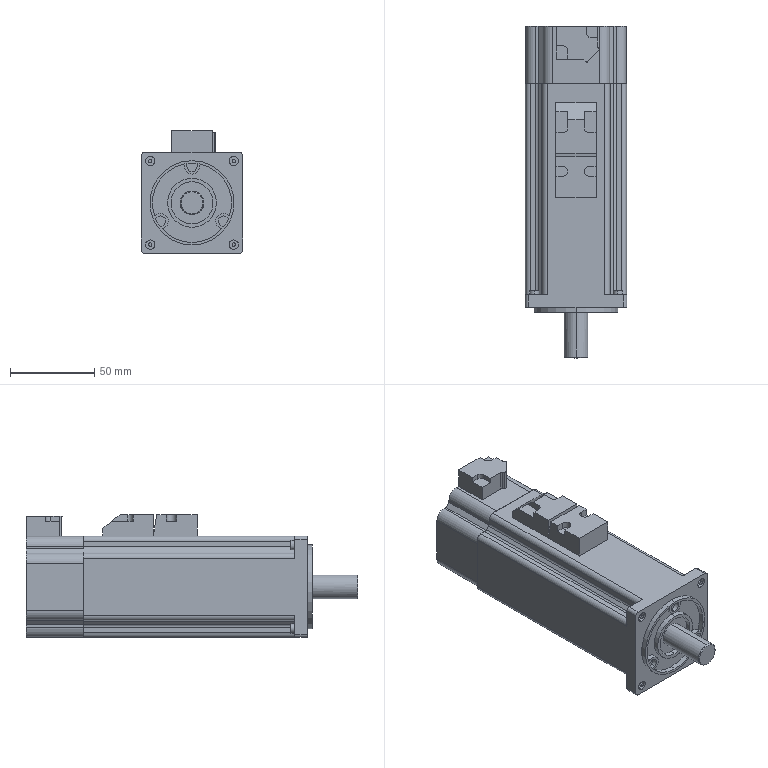Part | SolidWorks | features BaseBody 1 | 1 solid | 233 faces | box 60 x 196.8 x 72.85 mm | volume 561117 mm3 | plane 136 | cylinder 87 | cone 10 | commonest cylinder face diameters 6 x19 5.5 x16 2 x13 4 x12 12 x8 47 x7